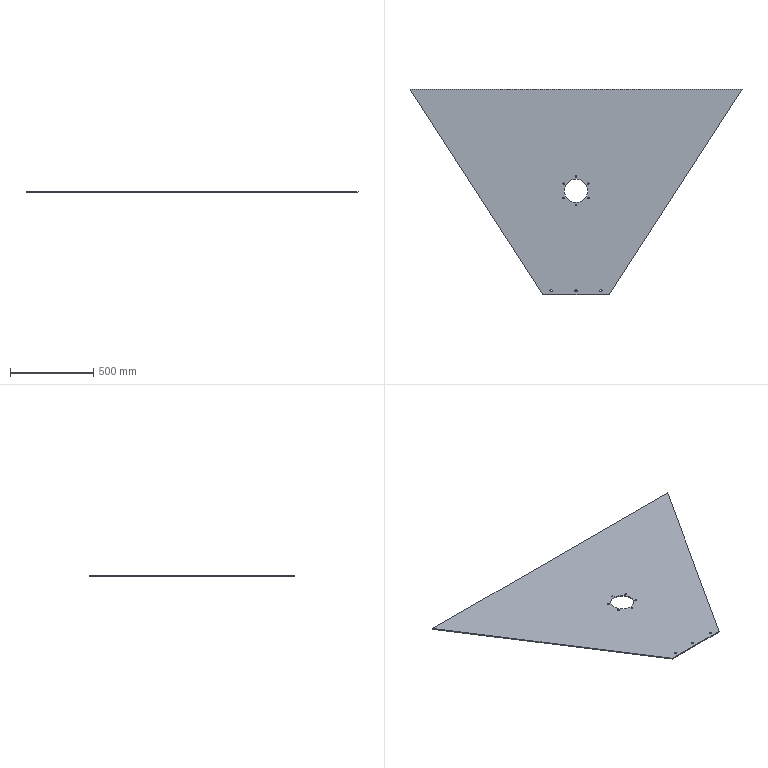Part | SolidWorks | features ICE 3, CirPattern 1, FlatPattern 1, SMBaseFlange 1, SheetMetal 1 | 1 solid | 26 faces | box 2000 x 1240 x 6 mm | volume 8830039 mm3 | cylinder 20 | plane 6 | commonest cylinder face diameters 10 x12 14 x6 140 x2
STEP:
#1=CARTESIAN_POINT('',(-68.612,49.5,-6.));
#2=VERTEX_POINT('',#1);
#3=CARTESIAN_POINT('',(-78.612,49.5,-6.));
#4=VERTEX_POINT('',#3);
#5=CARTESIAN_POINT('',(-73.612,49.5,-6.));
#6=DIRECTION('',(0.,0.,-1.));
#7=DIRECTION('',(1.,0.,0.));
#8=AXIS2_PLACEMENT_3D('',#5,#6,#7);
#9=CIRCLE('',#8,5.);
#10=EDGE_CURVE('',#2,#4,#9,.T.);
#11=ORIENTED_EDGE('',*,*,#10,.T.);
#12=CARTESIAN_POINT('',(-78.612,49.5,0.));
#13=VERTEX_POINT('',#12);
#14=CARTESIAN_POINT('',(-78.612,49.5,-6.001));
#15=DIRECTION('',(0.,0.,1.));
#16=VECTOR('',#15,1000.);
#17=LINE('',#14,#16);
#18=EDGE_CURVE('',#4,#13,#17,.T.);
#19=ORIENTED_EDGE('',*,*,#18,.T.);
#20=CARTESIAN_POINT('',(-68.612,49.5,0.));
#21=VERTEX_POINT('',#20);
#22=CARTESIAN_POINT('',(-73.612,49.5,0.));
#23=DIRECTION('',(0.,0.,1.));
#24=DIRECTION('',(0.5,0.866,0.));
#25=AXIS2_PLACEMENT_3D('',#22,#23,#24);
#26=CIRCLE('',#25,5.);
#27=EDGE_CURVE('',#13,#21,#26,.T.);
#28=ORIENTED_EDGE('',*,*,#27,.T.);
#29=CARTESIAN_POINT('',(-68.612,49.5,-6.001));
#30=DIRECTION('',(0.,0.,1.));
#31=VECTOR('',#30,1000.);
#32=LINE('',#29,#31);
#33=EDGE_CURVE('',#2,#21,#32,.T.);
#34=ORIENTED_EDGE('',*,*,#33,.F.);
#35=EDGE_LOOP('',(#11,#19,#28,#34));
#36=FACE_OUTER_BOUND('',#35,.T.);
#37=CARTESIAN_POINT('',(-73.612,49.5,-6.001));
#38=DIRECTION('',(0.,0.,1.));
#39=DIRECTION('',(1.,0.,0.));
#40=AXIS2_PLACEMENT_3D('',#37,#38,#39);
#41=CYLINDRICAL_SURFACE('',#40,5.);
#42=ADVANCED_FACE('',(#36),#41,.F.);
#43=CARTESIAN_POINT('',(-68.612,-35.5,-6.));
#44=VERTEX_POINT('',#43);
#45=CARTESIAN_POINT('',(-78.612,-35.5,-6.));
#46=VERTEX_POINT('',#45);
#47=CARTESIAN_POINT('',(-73.612,-35.5,-6.));
#48=DIRECTION('',(0.,0.,-1.));
#49=DIRECTION('',(1.,0.,0.));
#50=AXIS2_PLACEMENT_3D('',#47,#48,#49);
#51=CIRCLE('',#50,5.);
#52=EDGE_CURVE('',#44,#46,#51,.T.);
#53=ORIENTED_EDGE('',*,*,#52,.T.);
#54=CARTESIAN_POINT('',(-78.612,-35.5,0.));
#55=VERTEX_POINT('',#54);
#56=CARTESIAN_POINT('',(-78.612,-35.5,-6.001));
#57=DIRECTION('',(0.,0.,1.));
#58=VECTOR('',#57,1000.);
#59=LINE('',#56,#58);
#60=EDGE_CURVE('',#46,#55,#59,.T.);
#61=ORIENTED_EDGE('',*,*,#60,.T.);
#62=CARTESIAN_POINT('',(-68.612,-35.5,0.));
#63=VERTEX_POINT('',#62);
#64=CARTESIAN_POINT('',(-73.612,-35.5,0.));
#65=DIRECTION('',(0.,0.,1.));
#66=DIRECTION('',(-0.5,0.866,0.));
#67=AXIS2_PLACEMENT_3D('',#64,#65,#66);
#68=CIRCLE('',#67,5.);
#69=EDGE_CURVE('',#55,#63,#68,.T.);
#70=ORIENTED_EDGE('',*,*,#69,.T.);
#71=CARTESIAN_POINT('',(-68.612,-35.5,-6.001));
#72=DIRECTION('',(0.,0.,1.));
#73=VECTOR('',#72,1000.);
#74=LINE('',#71,#73);
#75=EDGE_CURVE('',#44,#63,#74,.T.);
#76=ORIENTED_EDGE('',*,*,#75,.F.);
#77=EDGE_LOOP('',(#53,#61,#70,#76));
#78=FACE_OUTER_BOUND('',#77,.T.);
#79=CARTESIAN_POINT('',(-73.612,-35.5,-6.001));
#80=DIRECTION('',(0.,0.,1.));
#81=DIRECTION('',(1.,0.,0.));
#82=AXIS2_PLACEMENT_3D('',#79,#80,#81);
#83=CYLINDRICAL_SURFACE('',#82,5.);
#84=ADVANCED_FACE('',(#78),#83,.F.);
#85=CARTESIAN_POINT('',(5.,-78.,-6.));
#86=VERTEX_POINT('',#85);
#87=CARTESIAN_POINT('',(-5.,-78.,-6.));
#88=VERTEX_POINT('',#87);
#89=CARTESIAN_POINT('',(0.,-78.,-6.));
#90=DIRECTION('',(0.,0.,-1.));
#91=DIRECTION('',(1.,0.,0.));
#92=AXIS2_PLACEMENT_3D('',#89,#90,#91);
#93=CIRCLE('',#92,5.);
#94=EDGE_CURVE('',#86,#88,#93,.T.);
#95=ORIENTED_EDGE('',*,*,#94,.T.);
#96=CARTESIAN_POINT('',(-5.,-78.,0.));
#97=VERTEX_POINT('',#96);
#98=CARTESIAN_POINT('',(-5.,-78.,-6.001));
#99=DIRECTION('',(0.,0.,1.));
#100=VECTOR('',#99,1000.);
#101=LINE('',#98,#100);
#102=EDGE_CURVE('',#88,#97,#101,.T.);
#103=ORIENTED_EDGE('',*,*,#102,.T.);
#104=CARTESIAN_POINT('',(5.,-78.,0.));
#105=VERTEX_POINT('',#104);
#106=CARTESIAN_POINT('',(0.,-78.,0.));
#107=DIRECTION('',(0.,0.,1.));
#108=DIRECTION('',(-1.,0.,0.));
#109=AXIS2_PLACEMENT_3D('',#106,#107,#108);
#110=CIRCLE('',#109,5.);
#111=EDGE_CURVE('',#97,#105,#110,.T.);
#112=ORIENTED_EDGE('',*,*,#111,.T.);
#113=CARTESIAN_POINT('',(5.,-78.,-6.001));
#114=DIRECTION('',(0.,0.,1.));
#115=VECTOR('',#114,1000.);
#116=LINE('',#113,#115);
#117=EDGE_CURVE('',#86,#105,#116,.T.);
#118=ORIENTED_EDGE('',*,*,#117,.F.);
#119=EDGE_LOOP('',(#95,#103,#112,#118));
#120=FACE_OUTER_BOUND('',#119,.T.);
#121=CARTESIAN_POINT('',(0.,-78.,-6.001));
#122=DIRECTION('',(0.,0.,1.));
#123=DIRECTION('',(1.,0.,0.));
#124=AXIS2_PLACEMENT_3D('',#121,#122,#123);
#125=CYLINDRICAL_SURFACE('',#124,5.);
#126=ADVANCED_FACE('',(#120),#125,.F.);
#127=CARTESIAN_POINT('',(78.612,-35.5,-6.));
#128=VERTEX_POINT('',#127);
#129=CARTESIAN_POINT('',(68.612,-35.5,-6.));
#130=VERTEX_POINT('',#129);
#131=CARTESIAN_POINT('',(73.612,-35.5,-6.));
#132=DIRECTION('',(0.,0.,-1.));
#133=DIRECTION('',(1.,0.,0.));
#134=AXIS2_PLACEMENT_3D('',#131,#132,#133);
#135=CIRCLE('',#134,5.);
#136=EDGE_CURVE('',#128,#130,#135,.T.);
#137=ORIENTED_EDGE('',*,*,#136,.T.);
#138=CARTESIAN_POINT('',(68.612,-35.5,0.));
#139=VERTEX_POINT('',#138);
#140=CARTESIAN_POINT('',(68.612,-35.5,-6.001));
#141=DIRECTION('',(0.,0.,1.));
#142=VECTOR('',#141,1000.);
#143=LINE('',#140,#142);
#144=EDGE_CURVE('',#130,#139,#143,.T.);
#145=ORIENTED_EDGE('',*,*,#144,.T.);
#146=CARTESIAN_POINT('',(78.612,-35.5,0.));
#147=VERTEX_POINT('',#146);
#148=CARTESIAN_POINT('',(73.612,-35.5,0.));
#149=DIRECTION('',(0.,0.,1.));
#150=DIRECTION('',(-0.5,-0.866,0.));
#151=AXIS2_PLACEMENT_3D('',#148,#149,#150);
#152=CIRCLE('',#151,5.);
#153=EDGE_CURVE('',#139,#147,#152,.T.);
#154=ORIENTED_EDGE('',*,*,#153,.T.);
#155=CARTESIAN_POINT('',(78.612,-35.5,-6.001));
#156=DIRECTION('',(0.,0.,1.));
#157=VECTOR('',#156,1000.);
#158=LINE('',#155,#157);
#159=EDGE_CURVE('',#128,#147,#158,.T.);
#160=ORIENTED_EDGE('',*,*,#159,.F.);
#161=EDGE_LOOP('',(#137,#145,#154,#160));
#162=FACE_OUTER_BOUND('',#161,.T.);
#163=CARTESIAN_POINT('',(73.612,-35.5,-6.001));
#164=DIRECTION('',(0.,0.,1.));
#165=DIRECTION('',(1.,0.,0.));
#166=AXIS2_PLACEMENT_3D('',#163,#164,#165);
#167=CYLINDRICAL_SURFACE('',#166,5.);
#168=ADVANCED_FACE('',(#162),#167,.F.);
#169=CARTESIAN_POINT('',(78.612,49.5,-6.));
#170=VERTEX_POINT('',#169);
#171=CARTESIAN_POINT('',(68.612,49.5,-6.));
#172=VERTEX_POINT('',#171);
#173=CARTESIAN_POINT('',(73.612,49.5,-6.));
#174=DIRECTION('',(0.,0.,-1.));
#175=DIRECTION('',(1.,0.,0.));
#176=AXIS2_PLACEMENT_3D('',#173,#174,#175);
#177=CIRCLE('',#176,5.);
#178=EDGE_CURVE('',#170,#172,#177,.T.);
#179=ORIENTED_EDGE('',*,*,#178,.T.);
#180=CARTESIAN_POINT('',(68.612,49.5,0.));
#181=VERTEX_POINT('',#180);
#182=CARTESIAN_POINT('',(68.612,49.5,-6.001));
#183=DIRECTION('',(0.,0.,1.));
#184=VECTOR('',#183,1000.);
#185=LINE('',#182,#184);
#186=EDGE_CURVE('',#172,#181,#185,.T.);
#187=ORIENTED_EDGE('',*,*,#186,.T.);
#188=CARTESIAN_POINT('',(78.612,49.5,0.));
#189=VERTEX_POINT('',#188);
#190=CARTESIAN_POINT('',(73.612,49.5,0.));
#191=DIRECTION('',(0.,0.,1.));
#192=DIRECTION('',(0.5,-0.866,0.));
#193=AXIS2_PLACEMENT_3D('',#190,#191,#192);
#194=CIRCLE('',#193,5.);
#195=EDGE_CURVE('',#181,#189,#194,.T.);
#196=ORIENTED_EDGE('',*,*,#195,.T.);
#197=CARTESIAN_POINT('',(78.612,49.5,-6.001));
#198=DIRECTION('',(0.,0.,1.));
#199=VECTOR('',#198,1000.);
#200=LINE('',#197,#199);
#201=EDGE_CURVE('',#170,#189,#200,.T.);
#202=ORIENTED_EDGE('',*,*,#201,.F.);
#203=EDGE_LOOP('',(#179,#187,#196,#202));
#204=FACE_OUTER_BOUND('',#203,.T.);
#205=CARTESIAN_POINT('',(73.612,49.5,-6.001));
#206=DIRECTION('',(0.,0.,1.));
#207=DIRECTION('',(1.,0.,0.));
#208=AXIS2_PLACEMENT_3D('',#205,#206,#207);
#209=CYLINDRICAL_SURFACE('',#208,5.);
#210=ADVANCED_FACE('',(#204),#209,.F.);
#211=CARTESIAN_POINT('',(-150.,-602.,0.));
#212=VERTEX_POINT('',#211);
#213=CARTESIAN_POINT('',(-150.,-588.,0.));
#214=VERTEX_POINT('',#213);
#215=CARTESIAN_POINT('',(-150.,-595.,0.));
#216=DIRECTION('',(0.,0.,-1.));
#217=DIRECTION('',(1.,0.,0.));
#218=AXIS2_PLACEMENT_3D('',#215,#216,#217);
#219=CIRCLE('',#218,7.);
#220=EDGE_CURVE('',#212,#214,#219,.T.);
#221=ORIENTED_EDGE('',*,*,#220,.F.);
#222=CARTESIAN_POINT('',(-150.,-602.,-6.));
#223=VERTEX_POINT('',#222);
#224=CARTESIAN_POINT('',(-150.,-602.,0.001));
#225=DIRECTION('',(0.,0.,-1.));
#226=VECTOR('',#225,1000.);
#227=LINE('',#224,#226);
#228=EDGE_CURVE('',#212,#223,#227,.T.);
#229=ORIENTED_EDGE('',*,*,#228,.T.);
#230=CARTESIAN_POINT('',(-150.,-588.,-6.));
#231=VERTEX_POINT('',#230);
#232=CARTESIAN_POINT('',(-150.,-595.,-6.));
#233=DIRECTION('',(0.,0.,-1.));
#234=DIRECTION('',(0.,1.,0.));
#235=AXIS2_PLACEMENT_3D('',#232,#233,#234);
#236=CIRCLE('',#235,7.);
#237=EDGE_CURVE('',#223,#231,#236,.T.);
#238=ORIENTED_EDGE('',*,*,#237,.T.);
#239=CARTESIAN_POINT('',(-150.,-588.,0.001));
#240=DIRECTION('',(0.,0.,-1.));
#241=VECTOR('',#240,1000.);
#242=LINE('',#239,#241);
#243=EDGE_CURVE('',#214,#231,#242,.T.);
#244=ORIENTED_EDGE('',*,*,#243,.F.);
#245=EDGE_LOOP('',(#221,#229,#238,#244));
#246=FACE_OUTER_BOUND('',#245,.T.);
#247=CARTESIAN_POINT('',(-150.,-595.,0.001));
#248=DIRECTION('',(0.,0.,-1.));
#249=DIRECTION('',(0.,1.,0.));
#250=AXIS2_PLACEMENT_3D('',#247,#248,#249);
#251=CYLINDRICAL_SURFACE('',#250,7.);
#252=ADVANCED_FACE('',(#246),#251,.F.);
#253=CARTESIAN_POINT('',(0.,-602.,0.));
#254=VERTEX_POINT('',#253);
#255=CARTESIAN_POINT('',(0.,-588.,0.));
#256=VERTEX_POINT('',#255);
#257=CARTESIAN_POINT('',(0.,-595.,0.));
#258=DIRECTION('',(0.,0.,-1.));
#259=DIRECTION('',(1.,0.,0.));
#260=AXIS2_PLACEMENT_3D('',#257,#258,#259);
#261=CIRCLE('',#260,7.);
#262=EDGE_CURVE('',#254,#256,#261,.T.);
#263=ORIENTED_EDGE('',*,*,#262,.F.);
#264=CARTESIAN_POINT('',(0.,-602.,-6.));
#265=VERTEX_POINT('',#264);
#266=CARTESIAN_POINT('',(0.,-602.,0.001));
#267=DIRECTION('',(0.,0.,-1.));
#268=VECTOR('',#267,1000.);
#269=LINE('',#266,#268);
#270=EDGE_CURVE('',#254,#265,#269,.T.);
#271=ORIENTED_EDGE('',*,*,#270,.T.);
#272=CARTESIAN_POINT('',(0.,-588.,-6.));
#273=VERTEX_POINT('',#272);
#274=CARTESIAN_POINT('',(0.,-595.,-6.));
#275=DIRECTION('',(0.,0.,-1.));
#276=DIRECTION('',(0.,1.,0.));
#277=AXIS2_PLACEMENT_3D('',#274,#275,#276);
#278=CIRCLE('',#277,7.);
#279=EDGE_CURVE('',#265,#273,#278,.T.);
#280=ORIENTED_EDGE('',*,*,#279,.T.);
#281=CARTESIAN_POINT('',(0.,-588.,0.001));
#282=DIRECTION('',(0.,0.,-1.));
#283=VECTOR('',#282,1000.);
#284=LINE('',#281,#283);
#285=EDGE_CURVE('',#256,#273,#284,.T.);
#286=ORIENTED_EDGE('',*,*,#285,.F.);
#287=EDGE_LOOP('',(#263,#271,#280,#286));
#288=FACE_OUTER_BOUND('',#287,.T.);
#289=CARTESIAN_POINT('',(0.,-595.,0.001));
#290=DIRECTION('',(0.,0.,-1.));
#291=DIRECTION('',(0.,1.,0.));
#292=AXIS2_PLACEMENT_3D('',#289,#290,#291);
#293=CYLINDRICAL_SURFACE('',#292,7.);
#294=ADVANCED_FACE('',(#288),#293,.F.);
#295=CARTESIAN_POINT('',(150.,-602.,0.));
#296=VERTEX_POINT('',#295);
#297=CARTESIAN_POINT('',(150.,-588.,0.));
#298=VERTEX_POINT('',#297);
#299=CARTESIAN_POINT('',(150.,-595.,0.));
#300=DIRECTION('',(0.,0.,-1.));
#301=DIRECTION('',(1.,0.,0.));
#302=AXIS2_PLACEMENT_3D('',#299,#300,#301);
#303=CIRCLE('',#302,7.);
#304=EDGE_CURVE('',#296,#298,#303,.T.);
#305=ORIENTED_EDGE('',*,*,#304,.F.);
#306=CARTESIAN_POINT('',(150.,-602.,-6.));
#307=VERTEX_POINT('',#306);
#308=CARTESIAN_POINT('',(150.,-602.,0.001));
#309=DIRECTION('',(0.,0.,-1.));
#310=VECTOR('',#309,1000.);
#311=LINE('',#308,#310);
#312=EDGE_CURVE('',#296,#307,#311,.T.);
#313=ORIENTED_EDGE('',*,*,#312,.T.);
#314=CARTESIAN_POINT('',(150.,-588.,-6.));
#315=VERTEX_POINT('',#314);
#316=CARTESIAN_POINT('',(150.,-595.,-6.));
#317=DIRECTION('',(0.,0.,-1.));
#318=DIRECTION('',(0.,1.,0.));
#319=AXIS2_PLACEMENT_3D('',#316,#317,#318);
#320=CIRCLE('',#319,7.);
#321=EDGE_CURVE('',#307,#315,#320,.T.);
#322=ORIENTED_EDGE('',*,*,#321,.T.);
#323=CARTESIAN_POINT('',(150.,-588.,0.001));
#324=DIRECTION('',(0.,0.,-1.));
#325=VECTOR('',#324,1000.);
#326=LINE('',#323,#325);
#327=EDGE_CURVE('',#298,#315,#326,.T.);
#328=ORIENTED_EDGE('',*,*,#327,.F.);
#329=EDGE_LOOP('',(#305,#313,#322,#328));
#330=FACE_OUTER_BOUND('',#329,.T.);
#331=CARTESIAN_POINT('',(150.,-595.,0.001));
#332=DIRECTION('',(0.,0.,-1.));
#333=DIRECTION('',(0.,1.,0.));
#334=AXIS2_PLACEMENT_3D('',#331,#332,#333);
#335=CYLINDRICAL_SURFACE('',#334,7.);
#336=ADVANCED_FACE('',(#330),#335,.F.);
#337=CARTESIAN_POINT('',(5.,92.,-6.));
#338=VERTEX_POINT('',#337);
#339=CARTESIAN_POINT('',(-5.,92.,-6.));
#340=VERTEX_POINT('',#339);
#341=CARTESIAN_POINT('',(0.,92.,-6.));
#342=DIRECTION('',(0.,0.,-1.));
#343=DIRECTION('',(1.,0.,0.));
#344=AXIS2_PLACEMENT_3D('',#341,#342,#343);
#345=CIRCLE('',#344,5.);
#346=EDGE_CURVE('',#338,#340,#345,.T.);
#347=ORIENTED_EDGE('',*,*,#346,.T.);
#348=CARTESIAN_POINT('',(-5.,92.,0.));
#349=VERTEX_POINT('',#348);
#350=CARTESIAN_POINT('',(-5.,92.,-6.001));
#351=DIRECTION('',(0.,0.,1.));
#352=VECTOR('',#351,1000.);
#353=LINE('',#350,#352);
#354=EDGE_CURVE('',#340,#349,#353,.T.);
#355=ORIENTED_EDGE('',*,*,#354,.T.);
#356=CARTESIAN_POINT('',(5.,92.,0.));
#357=VERTEX_POINT('',#356);
#358=CARTESIAN_POINT('',(0.,92.,0.));
#359=DIRECTION('',(0.,0.,1.));
#360=DIRECTION('',(1.,0.,0.));
#361=AXIS2_PLACEMENT_3D('',#358,#359,#360);
#362=CIRCLE('',#361,5.);
#363=EDGE_CURVE('',#349,#357,#362,.T.);
#364=ORIENTED_EDGE('',*,*,#363,.T.);
#365=CARTESIAN_POINT('',(5.,92.,-6.001));
#366=DIRECTION('',(0.,0.,1.));
#367=VECTOR('',#366,1000.);
#368=LINE('',#365,#367);
#369=EDGE_CURVE('',#338,#357,#368,.T.);
#370=ORIENTED_EDGE('',*,*,#369,.F.);
#371=EDGE_LOOP('',(#347,#355,#364,#370));
#372=FACE_OUTER_BOUND('',#371,.T.);
#373=CARTESIAN_POINT('',(0.,92.,-6.001));
#374=DIRECTION('',(0.,0.,1.));
#375=DIRECTION('',(1.,0.,0.));
#376=AXIS2_PLACEMENT_3D('',#373,#374,#375);
#377=CYLINDRICAL_SURFACE('',#376,5.);
#378=ADVANCED_FACE('',(#372),#377,.F.);
#379=CARTESIAN_POINT('',(70.,7.,-6.));
#380=VERTEX_POINT('',#379);
#381=CARTESIAN_POINT('',(-70.,7.,-6.));
#382=VERTEX_POINT('',#381);
#383=CARTESIAN_POINT('',(0.,7.,-6.));
#384=DIRECTION('',(0.,0.,-1.));
#385=DIRECTION('',(1.,0.,0.));
#386=AXIS2_PLACEMENT_3D('',#383,#384,#385);
#387=CIRCLE('',#386,70.);
#388=EDGE_CURVE('',#380,#382,#387,.T.);
#389=ORIENTED_EDGE('',*,*,#388,.T.);
#390=CARTESIAN_POINT('',(-70.,7.,0.));
#391=VERTEX_POINT('',#390);
#392=CARTESIAN_POINT('',(-70.,7.,-6.001));
#393=DIRECTION('',(0.,0.,1.));
#394=VECTOR('',#393,1000.);
#395=LINE('',#392,#394);
#396=EDGE_CURVE('',#382,#391,#395,.T.);
#397=ORIENTED_EDGE('',*,*,#396,.T.);
#398=CARTESIAN_POINT('',(70.,7.,0.));
#399=VERTEX_POINT('',#398);
#400=CARTESIAN_POINT('',(0.,7.,0.));
#401=DIRECTION('',(0.,0.,1.));
#402=DIRECTION('',(1.,0.,0.));
#403=AXIS2_PLACEMENT_3D('',#400,#401,#402);
#404=CIRCLE('',#403,70.);
#405=EDGE_CURVE('',#391,#399,#404,.T.);
#406=ORIENTED_EDGE('',*,*,#405,.T.);
#407=CARTESIAN_POINT('',(70.,7.,-6.001));
#408=DIRECTION('',(0.,0.,1.));
#409=VECTOR('',#408,1000.);
#410=LINE('',#407,#409);
#411=EDGE_CURVE('',#380,#399,#410,.T.);
#412=ORIENTED_EDGE('',*,*,#411,.F.);
#413=EDGE_LOOP('',(#389,#397,#406,#412));
#414=FACE_OUTER_BOUND('',#413,.T.);
#415=CARTESIAN_POINT('',(0.,7.,-6.001));
#416=DIRECTION('',(0.,0.,1.));
#417=DIRECTION('',(1.,0.,0.));
#418=AXIS2_PLACEMENT_3D('',#415,#416,#417);
#419=CYLINDRICAL_SURFACE('',#418,70.);
#420=ADVANCED_FACE('',(#414),#419,.F.);
#421=CARTESIAN_POINT('',(-200.,-620.,0.));
#422=VERTEX_POINT('',#421);
#423=CARTESIAN_POINT('',(200.,-620.,0.));
#424=VERTEX_POINT('',#423);
#425=CARTESIAN_POINT('',(1000.,-620.,0.));
#426=DIRECTION('',(1.,0.,0.));
#427=VECTOR('',#426,1000.);
#428=LINE('',#425,#427);
#429=EDGE_CURVE('',#422,#424,#428,.T.);
#430=ORIENTED_EDGE('',*,*,#429,.F.);
#431=CARTESIAN_POINT('',(-200.,-620.,-6.));
#432=VERTEX_POINT('',#431);
#433=CARTESIAN_POINT('',(-200.,-620.,-6.));
#434=DIRECTION('',(0.,0.,1.));
#435=VECTOR('',#434,1000.);
#436=LINE('',#433,#435);
#437=EDGE_CURVE('',#432,#422,#436,.T.);
#438=ORIENTED_EDGE('',*,*,#437,.F.);
#439=CARTESIAN_POINT('',(200.,-620.,-6.));
#440=VERTEX_POINT('',#439);
#441=CARTESIAN_POINT('',(1000.,-620.,-6.));
#442=DIRECTION('',(1.,0.,0.));
#443=VECTOR('',#442,1000.);
#444=LINE('',#441,#443);
#445=EDGE_CURVE('',#432,#440,#444,.T.);
#446=ORIENTED_EDGE('',*,*,#445,.T.);
#447=CARTESIAN_POINT('',(200.,-620.,-6.));
#448=DIRECTION('',(0.,0.,1.));
#449=VECTOR('',#448,1000.);
#450=LINE('',#447,#449);
#451=EDGE_CURVE('',#440,#424,#450,.T.);
#452=ORIENTED_EDGE('',*,*,#451,.T.);
#453=EDGE_LOOP('',(#430,#438,#446,#452));
#454=FACE_OUTER_BOUND('',#453,.T.);
#455=CARTESIAN_POINT('',(1000.,-620.,-6.));
#456=DIRECTION('',(0.,-1.,0.));
#457=DIRECTION('',(1.,0.,0.));
#458=AXIS2_PLACEMENT_3D('',#455,#456,#457);
#459=PLANE('',#458);
#460=ADVANCED_FACE('',(#454),#459,.T.);
#461=ORIENTED_EDGE('',*,*,#10,.F.);
#462=CARTESIAN_POINT('',(-73.612,49.5,-6.));
#463=DIRECTION('',(0.,0.,-1.));
#464=DIRECTION('',(1.,0.,0.));
#465=AXIS2_PLACEMENT_3D('',#462,#463,#464);
#466=CIRCLE('',#465,5.);
#467=EDGE_CURVE('',#4,#2,#466,.T.);
#468=ORIENTED_EDGE('',*,*,#467,.F.);
#469=EDGE_LOOP('',(#461,#468));
#470=FACE_BOUND('',#469,.T.);
#471=ORIENTED_EDGE('',*,*,#52,.F.);
#472=CARTESIAN_POINT('',(-73.612,-35.5,-6.));
#473=DIRECTION('',(0.,0.,-1.));
#474=DIRECTION('',(1.,0.,0.));
#475=AXIS2_PLACEMENT_3D('',#472,#473,#474);
#476=CIRCLE('',#475,5.);
#477=EDGE_CURVE('',#46,#44,#476,.T.);
#478=ORIENTED_EDGE('',*,*,#477,.F.);
#479=EDGE_LOOP('',(#471,#478));
#480=FACE_BOUND('',#479,.T.);
#481=ORIENTED_EDGE('',*,*,#94,.F.);
#482=CARTESIAN_POINT('',(0.,-78.,-6.));
#483=DIRECTION('',(0.,0.,-1.));
#484=DIRECTION('',(1.,0.,0.));
#485=AXIS2_PLACEMENT_3D('',#482,#483,#484);
#486=CIRCLE('',#485,5.);
#487=EDGE_CURVE('',#88,#86,#486,.T.);
#488=ORIENTED_EDGE('',*,*,#487,.F.);
#489=EDGE_LOOP('',(#481,#488));
#490=FACE_BOUND('',#489,.T.);
#491=ORIENTED_EDGE('',*,*,#136,.F.);
#492=CARTESIAN_POINT('',(73.612,-35.5,-6.));
#493=DIRECTION('',(0.,0.,-1.));
#494=DIRECTION('',(1.,0.,0.));
#495=AXIS2_PLACEMENT_3D('',#492,#493,#494);
#496=CIRCLE('',#495,5.);
#497=EDGE_CURVE('',#130,#128,#496,.T.);
#498=ORIENTED_EDGE('',*,*,#497,.F.);
#499=EDGE_LOOP('',(#491,#498));
#500=FACE_BOUND('',#499,.T.);
#501=ORIENTED_EDGE('',*,*,#178,.F.);
#502=CARTESIAN_POINT('',(73.612,49.5,-6.));
#503=DIRECTION('',(0.,0.,-1.));
#504=DIRECTION('',(1.,0.,0.));
#505=AXIS2_PLACEMENT_3D('',#502,#503,#504);
#506=CIRCLE('',#505,5.);
#507=EDGE_CURVE('',#172,#170,#506,.T.);
#508=ORIENTED_EDGE('',*,*,#507,.F.);
#509=EDGE_LOOP('',(#501,#508));
#510=FACE_BOUND('',#509,.T.);
#511=CARTESIAN_POINT('',(-150.,-595.,-6.));
#512=DIRECTION('',(0.,0.,-1.));
#513=DIRECTION('',(0.,1.,0.));
#514=AXIS2_PLACEMENT_3D('',#511,#512,#513);
#515=CIRCLE('',#514,7.);
#516=EDGE_CURVE('',#231,#223,#515,.T.);
#517=ORIENTED_EDGE('',*,*,#516,.F.);
#518=ORIENTED_EDGE('',*,*,#237,.F.);
#519=EDGE_LOOP('',(#517,#518));
#520=FACE_BOUND('',#519,.T.);
#521=CARTESIAN_POINT('',(0.,-595.,-6.));
#522=DIRECTION('',(0.,0.,-1.));
#523=DIRECTION('',(0.,1.,0.));
#524=AXIS2_PLACEMENT_3D('',#521,#522,#523);
#525=CIRCLE('',#524,7.);
#526=EDGE_CURVE('',#273,#265,#525,.T.);
#527=ORIENTED_EDGE('',*,*,#526,.F.);
#528=ORIENTED_EDGE('',*,*,#279,.F.);
#529=EDGE_LOOP('',(#527,#528));
#530=FACE_BOUND('',#529,.T.);
#531=CARTESIAN_POINT('',(150.,-595.,-6.));
#532=DIRECTION('',(0.,0.,-1.));
#533=DIRECTION('',(0.,1.,0.));
#534=AXIS2_PLACEMENT_3D('',#531,#532,#533);
#535=CIRCLE('',#534,7.);
#536=EDGE_CURVE('',#315,#307,#535,.T.);
#537=ORIENTED_EDGE('',*,*,#536,.F.);
#538=ORIENTED_EDGE('',*,*,#321,.F.);
#539=EDGE_LOOP('',(#537,#538));
#540=FACE_BOUND('',#539,.T.);
#541=ORIENTED_EDGE('',*,*,#346,.F.);
#542=CARTESIAN_POINT('',(0.,92.,-6.));
#543=DIRECTION('',(0.,0.,-1.));
#544=DIRECTION('',(1.,0.,0.));
#545=AXIS2_PLACEMENT_3D('',#542,#543,#544);
#546=CIRCLE('',#545,5.);
#547=EDGE_CURVE('',#340,#338,#546,.T.);
#548=ORIENTED_EDGE('',*,*,#547,.F.);
#549=EDGE_LOOP('',(#541,#548));
#550=FACE_BOUND('',#549,.T.);
#551=ORIENTED_EDGE('',*,*,#388,.F.);
#552=CARTESIAN_POINT('',(0.,7.,-6.));
#553=DIRECTION('',(0.,0.,-1.));
#554=DIRECTION('',(1.,0.,0.));
#555=AXIS2_PLACEMENT_3D('',#552,#553,#554);
#556=CIRCLE('',#555,70.);
#557=EDGE_CURVE('',#382,#380,#556,.T.);
#558=ORIENTED_EDGE('',*,*,#557,.F.);
#559=EDGE_LOOP('',(#551,#558));
#560=FACE_BOUND('',#559,.T.);
#561=CARTESIAN_POINT('',(-1000.,620.,-6.));
#562=VERTEX_POINT('',#561);
#563=CARTESIAN_POINT('',(-1000.,620.,-6.));
#564=DIRECTION('',(0.5421,-0.8403,0.));
#565=VECTOR('',#564,1000.);
#566=LINE('',#563,#565);
#567=EDGE_CURVE('',#562,#432,#566,.T.);
#568=ORIENTED_EDGE('',*,*,#567,.F.);
#569=CARTESIAN_POINT('',(1000.,620.,-6.));
#570=VERTEX_POINT('',#569);
#571=CARTESIAN_POINT('',(1000.,620.,-6.));
#572=DIRECTION('',(-1.,0.,0.));
#573=VECTOR('',#572,1000.);
#574=LINE('',#571,#573);
#575=EDGE_CURVE('',#570,#562,#574,.T.);
#576=ORIENTED_EDGE('',*,*,#575,.F.);
#577=CARTESIAN_POINT('',(1000.,620.,-6.));
#578=DIRECTION('',(0.5421,0.8403,0.));
#579=VECTOR('',#578,1000.);
#580=LINE('',#577,#579);
#581=EDGE_CURVE('',#440,#570,#580,.T.);
#582=ORIENTED_EDGE('',*,*,#581,.F.);
#583=ORIENTED_EDGE('',*,*,#445,.F.);
#584=EDGE_LOOP('',(#568,#576,#582,#583));
#585=FACE_OUTER_BOUND('',#584,.T.);
#586=CARTESIAN_POINT('',(0.,0.,-6.));
#587=DIRECTION('',(0.,0.,1.));
#588=DIRECTION('',(1.,0.,0.));
#589=AXIS2_PLACEMENT_3D('',#586,#587,#588);
#590=PLANE('',#589);
#591=ADVANCED_FACE('',(#470,#480,#490,#500,#510,#520,#530,#540,#550,#560,#585),#590,.F.);
#592=CARTESIAN_POINT('',(-73.612,49.5,0.));
#593=DIRECTION('',(0.,0.,1.));
#594=DIRECTION('',(0.5,0.866,0.));
#595=AXIS2_PLACEMENT_3D('',#592,#593,#594);
#596=CIRCLE('',#595,5.);
#597=EDGE_CURVE('',#21,#13,#596,.T.);
#598=ORIENTED_EDGE('',*,*,#597,.F.);
#599=ORIENTED_EDGE('',*,*,#27,.F.);
#600=EDGE_LOOP('',(#598,#599));
#601=FACE_BOUND('',#600,.T.);
#602=CARTESIAN_POINT('',(-73.612,-35.5,0.));
#603=DIRECTION('',(0.,0.,1.));
#604=DIRECTION('',(-0.5,0.866,0.));
#605=AXIS2_PLACEMENT_3D('',#602,#603,#604);
#606=CIRCLE('',#605,5.);
#607=EDGE_CURVE('',#63,#55,#606,.T.);
#608=ORIENTED_EDGE('',*,*,#607,.F.);
#609=ORIENTED_EDGE('',*,*,#69,.F.);
#610=EDGE_LOOP('',(#608,#609));
#611=FACE_BOUND('',#610,.T.);
#612=CARTESIAN_POINT('',(0.,-78.,0.));
#613=DIRECTION('',(0.,0.,1.));
#614=DIRECTION('',(-1.,0.,0.));
#615=AXIS2_PLACEMENT_3D('',#612,#613,#614);
#616=CIRCLE('',#615,5.);
#617=EDGE_CURVE('',#105,#97,#616,.T.);
#618=ORIENTED_EDGE('',*,*,#617,.F.);
#619=ORIENTED_EDGE('',*,*,#111,.F.);
#620=EDGE_LOOP('',(#618,#619));
#621=FACE_BOUND('',#620,.T.);
#622=CARTESIAN_POINT('',(73.612,-35.5,0.));
#623=DIRECTION('',(0.,0.,1.));
#624=DIRECTION('',(-0.5,-0.866,0.));
#625=AXIS2_PLACEMENT_3D('',#622,#623,#624);
#626=CIRCLE('',#625,5.);
#627=EDGE_CURVE('',#147,#139,#626,.T.);
#628=ORIENTED_EDGE('',*,*,#627,.F.);
#629=ORIENTED_EDGE('',*,*,#153,.F.);
#630=EDGE_LOOP('',(#628,#629));
#631=FACE_BOUND('',#630,.T.);
#632=CARTESIAN_POINT('',(73.612,49.5,0.));
#633=DIRECTION('',(0.,0.,1.));
#634=DIRECTION('',(0.5,-0.866,0.));
#635=AXIS2_PLACEMENT_3D('',#632,#633,#634);
#636=CIRCLE('',#635,5.);
#637=EDGE_CURVE('',#189,#181,#636,.T.);
#638=ORIENTED_EDGE('',*,*,#637,.F.);
#639=ORIENTED_EDGE('',*,*,#195,.F.);
#640=EDGE_LOOP('',(#638,#639));
#641=FACE_BOUND('',#640,.T.);
#642=CARTESIAN_POINT('',(-150.,-595.,0.));
#643=DIRECTION('',(0.,0.,-1.));
#644=DIRECTION('',(1.,0.,0.));
#645=AXIS2_PLACEMENT_3D('',#642,#643,#644);
#646=CIRCLE('',#645,7.);
#647=EDGE_CURVE('',#214,#212,#646,.T.);
#648=ORIENTED_EDGE('',*,*,#647,.T.);
#649=ORIENTED_EDGE('',*,*,#220,.T.);
#650=EDGE_LOOP('',(#648,#649));
#651=FACE_BOUND('',#650,.T.);
#652=CARTESIAN_POINT('',(0.,-595.,0.));
#653=DIRECTION('',(0.,0.,-1.));
#654=DIRECTION('',(1.,0.,0.));
#655=AXIS2_PLACEMENT_3D('',#652,#653,#654);
#656=CIRCLE('',#655,7.);
#657=EDGE_CURVE('',#256,#254,#656,.T.);
#658=ORIENTED_EDGE('',*,*,#657,.T.);
#659=ORIENTED_EDGE('',*,*,#262,.T.);
#660=EDGE_LOOP('',(#658,#659));
#661=FACE_BOUND('',#660,.T.);
#662=CARTESIAN_POINT('',(150.,-595.,0.));
#663=DIRECTION('',(0.,0.,-1.));
#664=DIRECTION('',(1.,0.,0.));
#665=AXIS2_PLACEMENT_3D('',#662,#663,#664);
#666=CIRCLE('',#665,7.);
#667=EDGE_CURVE('',#298,#296,#666,.T.);
#668=ORIENTED_EDGE('',*,*,#667,.T.);
#669=ORIENTED_EDGE('',*,*,#304,.T.);
#670=EDGE_LOOP('',(#668,#669));
#671=FACE_BOUND('',#670,.T.);
#672=CARTESIAN_POINT('',(0.,92.,0.));
#673=DIRECTION('',(0.,0.,1.));
#674=DIRECTION('',(1.,0.,0.));
#675=AXIS2_PLACEMENT_3D('',#672,#673,#674);
#676=CIRCLE('',#675,5.);
#677=EDGE_CURVE('',#357,#349,#676,.T.);
#678=ORIENTED_EDGE('',*,*,#677,.F.);
#679=ORIENTED_EDGE('',*,*,#363,.F.);
#680=EDGE_LOOP('',(#678,#679));
#681=FACE_BOUND('',#680,.T.);
#682=CARTESIAN_POINT('',(0.,7.,0.));
#683=DIRECTION('',(0.,0.,1.));
#684=DIRECTION('',(1.,0.,0.));
#685=AXIS2_PLACEMENT_3D('',#682,#683,#684);
#686=CIRCLE('',#685,70.);
#687=EDGE_CURVE('',#399,#391,#686,.T.);
#688=ORIENTED_EDGE('',*,*,#687,.F.);
#689=ORIENTED_EDGE('',*,*,#405,.F.);
#690=EDGE_LOOP('',(#688,#689));
#691=FACE_BOUND('',#690,.T.);
#692=CARTESIAN_POINT('',(1000.,620.,0.));
#693=VERTEX_POINT('',#692);
#694=CARTESIAN_POINT('',(-1000.,620.,0.));
#695=VERTEX_POINT('',#694);
#696=CARTESIAN_POINT('',(1000.,620.,0.));
#697=DIRECTION('',(-1.,0.,0.));
#698=VECTOR('',#697,1000.);
#699=LINE('',#696,#698);
#700=EDGE_CURVE('',#693,#695,#699,.T.);
#701=ORIENTED_EDGE('',*,*,#700,.T.);
#702=CARTESIAN_POINT('',(-1000.,620.,0.));
#703=DIRECTION('',(0.5421,-0.8403,0.));
#704=VECTOR('',#703,1000.);
#705=LINE('',#702,#704);
#706=EDGE_CURVE('',#695,#422,#705,.T.);
#707=ORIENTED_EDGE('',*,*,#706,.T.);
#708=ORIENTED_EDGE('',*,*,#429,.T.);
#709=CARTESIAN_POINT('',(1000.,620.,0.));
#710=DIRECTION('',(0.5421,0.8403,0.));
#711=VECTOR('',#710,1000.);
#712=LINE('',#709,#711);
#713=EDGE_CURVE('',#424,#693,#712,.T.);
#714=ORIENTED_EDGE('',*,*,#713,.T.);
#715=EDGE_LOOP('',(#701,#707,#708,#714));
#716=FACE_OUTER_BOUND('',#715,.T.);
#717=CARTESIAN_POINT('',(0.,0.,0.));
#718=DIRECTION('',(0.,0.,1.));
#719=DIRECTION('',(1.,0.,0.));
#720=AXIS2_PLACEMENT_3D('',#717,#718,#719);
#721=PLANE('',#720);
#722=ADVANCED_FACE('',(#601,#611,#621,#631,#641,#651,#661,#671,#681,#691,#716),#721,.T.);
#723=ORIENTED_EDGE('',*,*,#700,.F.);
#724=CARTESIAN_POINT('',(1000.,620.,-6.));
#725=DIRECTION('',(0.,0.,1.));
#726=VECTOR('',#725,1000.);
#727=LINE('',#724,#726);
#728=EDGE_CURVE('',#570,#693,#727,.T.);
#729=ORIENTED_EDGE('',*,*,#728,.F.);
#730=ORIENTED_EDGE('',*,*,#575,.T.);
#731=CARTESIAN_POINT('',(-1000.,620.,-6.));
#732=DIRECTION('',(0.,0.,1.));
#733=VECTOR('',#732,1000.);
#734=LINE('',#731,#733);
#735=EDGE_CURVE('',#562,#695,#734,.T.);
#736=ORIENTED_EDGE('',*,*,#735,.T.);
#737=EDGE_LOOP('',(#723,#729,#730,#736));
#738=FACE_OUTER_BOUND('',#737,.T.);
#739=CARTESIAN_POINT('',(1000.,620.,-6.));
#740=DIRECTION('',(0.,1.,0.));
#741=DIRECTION('',(-1.,0.,0.));
#742=AXIS2_PLACEMENT_3D('',#739,#740,#741);
#743=PLANE('',#742);
#744=ADVANCED_FACE('',(#738),#743,.T.);
#745=ORIENTED_EDGE('',*,*,#451,.F.);
#746=ORIENTED_EDGE('',*,*,#581,.T.);
#747=ORIENTED_EDGE('',*,*,#728,.T.);
#748=ORIENTED_EDGE('',*,*,#713,.F.);
#749=EDGE_LOOP('',(#745,#746,#747,#748));
#750=FACE_OUTER_BOUND('',#749,.T.);
#751=CARTESIAN_POINT('',(1000.,620.,-6.));
#752=DIRECTION('',(0.8403,-0.5421,0.));
#753=DIRECTION('',(0.5421,0.8403,0.));
#754=AXIS2_PLACEMENT_3D('',#751,#752,#753);
#755=PLANE('',#754);
#756=ADVANCED_FACE('',(#750),#755,.T.);
#757=ORIENTED_EDGE('',*,*,#735,.F.);
#758=ORIENTED_EDGE('',*,*,#567,.T.);
#759=ORIENTED_EDGE('',*,*,#437,.T.);
#760=ORIENTED_EDGE('',*,*,#706,.F.);
#761=EDGE_LOOP('',(#757,#758,#759,#760));
#762=FACE_OUTER_BOUND('',#761,.T.);
#763=CARTESIAN_POINT('',(-1000.,620.,-6.));
#764=DIRECTION('',(-0.8403,-0.5421,0.));
#765=DIRECTION('',(0.5421,-0.8403,0.));
#766=AXIS2_PLACEMENT_3D('',#763,#764,#765);
#767=PLANE('',#766);
#768=ADVANCED_FACE('',(#762),#767,.T.);
#769=ORIENTED_EDGE('',*,*,#396,.F.);
#770=ORIENTED_EDGE('',*,*,#557,.T.);
#771=ORIENTED_EDGE('',*,*,#411,.T.);
#772=ORIENTED_EDGE('',*,*,#687,.T.);
#773=EDGE_LOOP('',(#769,#770,#771,#772));
#774=FACE_OUTER_BOUND('',#773,.T.);
#775=CARTESIAN_POINT('',(0.,7.,-6.001));
#776=DIRECTION('',(0.,0.,1.));
#777=DIRECTION('',(1.,0.,0.));
#778=AXIS2_PLACEMENT_3D('',#775,#776,#777);
#779=CYLINDRICAL_SURFACE('',#778,70.);
#780=ADVANCED_FACE('',(#774),#779,.F.);
#781=ORIENTED_EDGE('',*,*,#354,.F.);
#782=ORIENTED_EDGE('',*,*,#547,.T.);
#783=ORIENTED_EDGE('',*,*,#369,.T.);
#784=ORIENTED_EDGE('',*,*,#677,.T.);
#785=EDGE_LOOP('',(#781,#782,#783,#784));
#786=FACE_OUTER_BOUND('',#785,.T.);
#787=CARTESIAN_POINT('',(0.,92.,-6.001));
#788=DIRECTION('',(0.,0.,1.));
#789=DIRECTION('',(1.,0.,0.));
#790=AXIS2_PLACEMENT_3D('',#787,#788,#789);
#791=CYLINDRICAL_SURFACE('',#790,5.);
#792=ADVANCED_FACE('',(#786),#791,.F.);
#793=ORIENTED_EDGE('',*,*,#312,.F.);
#794=ORIENTED_EDGE('',*,*,#667,.F.);
#795=ORIENTED_EDGE('',*,*,#327,.T.);
#796=ORIENTED_EDGE('',*,*,#536,.T.);
#797=EDGE_LOOP('',(#793,#794,#795,#796));
#798=FACE_OUTER_BOUND('',#797,.T.);
#799=CARTESIAN_POINT('',(150.,-595.,0.001));
#800=DIRECTION('',(0.,0.,-1.));
#801=DIRECTION('',(0.,1.,0.));
#802=AXIS2_PLACEMENT_3D('',#799,#800,#801);
#803=CYLINDRICAL_SURFACE('',#802,7.);
#804=ADVANCED_FACE('',(#798),#803,.F.);
#805=ORIENTED_EDGE('',*,*,#270,.F.);
#806=ORIENTED_EDGE('',*,*,#657,.F.);
#807=ORIENTED_EDGE('',*,*,#285,.T.);
#808=ORIENTED_EDGE('',*,*,#526,.T.);
#809=EDGE_LOOP('',(#805,#806,#807,#808));
#810=FACE_OUTER_BOUND('',#809,.T.);
#811=CARTESIAN_POINT('',(0.,-595.,0.001));
#812=DIRECTION('',(0.,0.,-1.));
#813=DIRECTION('',(0.,1.,0.));
#814=AXIS2_PLACEMENT_3D('',#811,#812,#813);
#815=CYLINDRICAL_SURFACE('',#814,7.);
#816=ADVANCED_FACE('',(#810),#815,.F.);
#817=ORIENTED_EDGE('',*,*,#228,.F.);
#818=ORIENTED_EDGE('',*,*,#647,.F.);
#819=ORIENTED_EDGE('',*,*,#243,.T.);
#820=ORIENTED_EDGE('',*,*,#516,.T.);
#821=EDGE_LOOP('',(#817,#818,#819,#820));
#822=FACE_OUTER_BOUND('',#821,.T.);
#823=CARTESIAN_POINT('',(-150.,-595.,0.001));
#824=DIRECTION('',(0.,0.,-1.));
#825=DIRECTION('',(0.,1.,0.));
#826=AXIS2_PLACEMENT_3D('',#823,#824,#825);
#827=CYLINDRICAL_SURFACE('',#826,7.);
#828=ADVANCED_FACE('',(#822),#827,.F.);
#829=ORIENTED_EDGE('',*,*,#186,.F.);
#830=ORIENTED_EDGE('',*,*,#507,.T.);
#831=ORIENTED_EDGE('',*,*,#201,.T.);
#832=ORIENTED_EDGE('',*,*,#637,.T.);
#833=EDGE_LOOP('',(#829,#830,#831,#832));
#834=FACE_OUTER_BOUND('',#833,.T.);
#835=CARTESIAN_POINT('',(73.612,49.5,-6.001));
#836=DIRECTION('',(0.,0.,1.));
#837=DIRECTION('',(1.,0.,0.));
#838=AXIS2_PLACEMENT_3D('',#835,#836,#837);
#839=CYLINDRICAL_SURFACE('',#838,5.);
#840=ADVANCED_FACE('',(#834),#839,.F.);
#841=ORIENTED_EDGE('',*,*,#144,.F.);
#842=ORIENTED_EDGE('',*,*,#497,.T.);
#843=ORIENTED_EDGE('',*,*,#159,.T.);
#844=ORIENTED_EDGE('',*,*,#627,.T.);
#845=EDGE_LOOP('',(#841,#842,#843,#844));
#846=FACE_OUTER_BOUND('',#845,.T.);
#847=CARTESIAN_POINT('',(73.612,-35.5,-6.001));
#848=DIRECTION('',(0.,0.,1.));
#849=DIRECTION('',(1.,0.,0.));
#850=AXIS2_PLACEMENT_3D('',#847,#848,#849);
#851=CYLINDRICAL_SURFACE('',#850,5.);
#852=ADVANCED_FACE('',(#846),#851,.F.);
#853=ORIENTED_EDGE('',*,*,#102,.F.);
#854=ORIENTED_EDGE('',*,*,#487,.T.);
#855=ORIENTED_EDGE('',*,*,#117,.T.);
#856=ORIENTED_EDGE('',*,*,#617,.T.);
#857=EDGE_LOOP('',(#853,#854,#855,#856));
#858=FACE_OUTER_BOUND('',#857,.T.);
#859=CARTESIAN_POINT('',(0.,-78.,-6.001));
#860=DIRECTION('',(0.,0.,1.));
#861=DIRECTION('',(1.,0.,0.));
#862=AXIS2_PLACEMENT_3D('',#859,#860,#861);
#863=CYLINDRICAL_SURFACE('',#862,5.);
#864=ADVANCED_FACE('',(#858),#863,.F.);
#865=ORIENTED_EDGE('',*,*,#60,.F.);
#866=ORIENTED_EDGE('',*,*,#477,.T.);
#867=ORIENTED_EDGE('',*,*,#75,.T.);
#868=ORIENTED_EDGE('',*,*,#607,.T.);
#869=EDGE_LOOP('',(#865,#866,#867,#868));
#870=FACE_OUTER_BOUND('',#869,.T.);
#871=CARTESIAN_POINT('',(-73.612,-35.5,-6.001));
#872=DIRECTION('',(0.,0.,1.));
#873=DIRECTION('',(1.,0.,0.));
#874=AXIS2_PLACEMENT_3D('',#871,#872,#873);
#875=CYLINDRICAL_SURFACE('',#874,5.);
#876=ADVANCED_FACE('',(#870),#875,.F.);
#877=ORIENTED_EDGE('',*,*,#18,.F.);
#878=ORIENTED_EDGE('',*,*,#467,.T.);
#879=ORIENTED_EDGE('',*,*,#33,.T.);
#880=ORIENTED_EDGE('',*,*,#597,.T.);
#881=EDGE_LOOP('',(#877,#878,#879,#880));
#882=FACE_OUTER_BOUND('',#881,.T.);
#883=CARTESIAN_POINT('',(-73.612,49.5,-6.001));
#884=DIRECTION('',(0.,0.,1.));
#885=DIRECTION('',(1.,0.,0.));
#886=AXIS2_PLACEMENT_3D('',#883,#884,#885);
#887=CYLINDRICAL_SURFACE('',#886,5.);
#888=ADVANCED_FACE('',(#882),#887,.F.);
#889=CLOSED_SHELL('',(#42,#84,#126,#168,#210,#252,#294,#336,#378,#420,#460,#591,#722,#744,#756,#768,#780,#792,#804,#816,#828,#840,#852,#864,#876,#888));
#890=MANIFOLD_SOLID_BREP('',#889);
#891=CARTESIAN_POINT('',(0.,0.,0.));
#892=DIRECTION('',(0.,0.,1.));
#893=DIRECTION('',(1.,0.,0.));
#894=AXIS2_PLACEMENT_3D('',#891,#892,#893);
#895=(LENGTH_UNIT()NAMED_UNIT(*)SI_UNIT(.MILLI.,.METRE.));
#896=UNCERTAINTY_MEASURE_WITH_UNIT(LENGTH_MEASURE(0.00001),#895,'','');
#897=(NAMED_UNIT(*)PLANE_ANGLE_UNIT()SI_UNIT($,.RADIAN.));
#898=(NAMED_UNIT(*)SI_UNIT($,.STERADIAN.)SOLID_ANGLE_UNIT());
#899=(GEOMETRIC_REPRESENTATION_CONTEXT(3)GLOBAL_UNCERTAINTY_ASSIGNED_CONTEXT((#896))GLOBAL_UNIT_ASSIGNED_CONTEXT((#895,#897,#898))REPRESENTATION_CONTEXT('',''));
#900=ADVANCED_BREP_SHAPE_REPRESENTATION('',(#890,#894),#899);